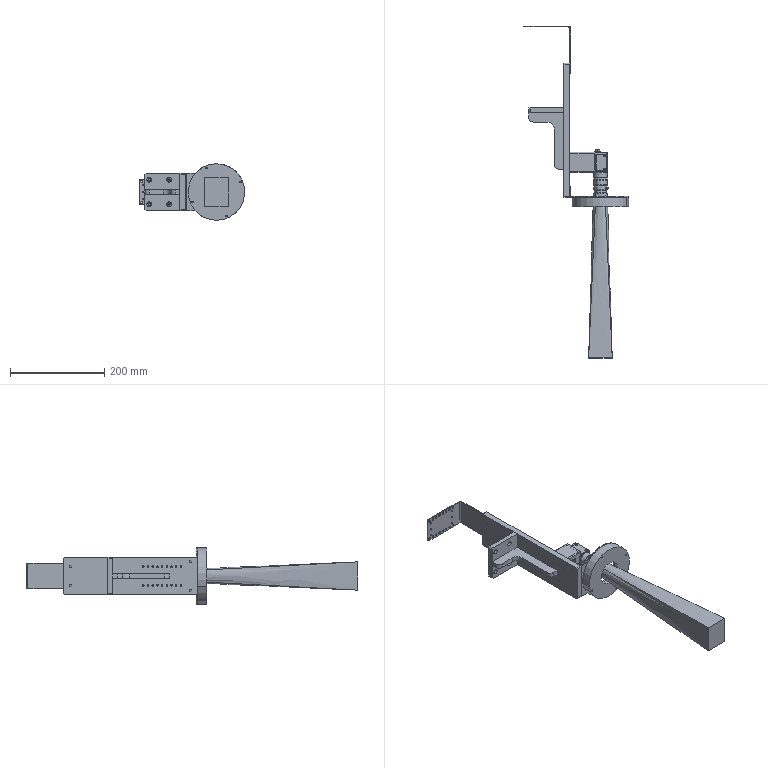Part | SolidWorks | features CompositeCurve 1 | 12 solids | 1559 faces | box 223.5 x 705 x 120 mm | volume 1273117 mm3 | plane 648 | cylinder 446 | spline 255 | cone 208 | torus 2 | commonest cylinder face diameters 3.3 x56 4.2 x44 3 x26 2 x22 3.4 x22 5.5 x20